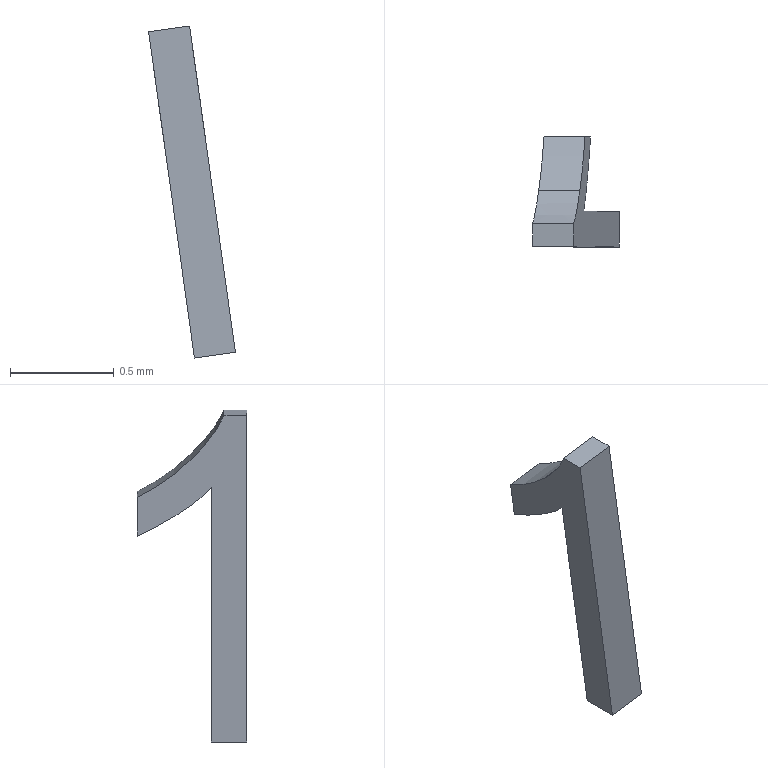Part | Creo | 1 solid | 11 faces | box 0.4191 x 0.529 x 1.601 mm | volume 0.06894 mm3 | plane 7 | other 4
STEP:
#1=CARTESIAN_POINT('',(-71.999,-126.498,-130.65));
#2=VERTEX_POINT('',#1);
#3=CARTESIAN_POINT('',(-72.171,-126.498,-129.425));
#4=VERTEX_POINT('',#3);
#5=CARTESIAN_POINT('',(-71.999,-126.498,-130.65));
#6=DIRECTION('',(-0.1392,0.,0.9903));
#7=VECTOR('',#6,1.237);
#8=LINE('',#5,#7);
#9=EDGE_CURVE('',#2,#4,#8,.T.);
#10=ORIENTED_EDGE('',*,*,#9,.F.);
#11=CARTESIAN_POINT('',(-71.801,-126.498,-130.622));
#12=VERTEX_POINT('',#11);
#13=CARTESIAN_POINT('',(-71.801,-126.498,-130.622));
#14=DIRECTION('',(-0.9903,0.,-0.1392));
#15=VECTOR('',#14,0.2);
#16=LINE('',#13,#15);
#17=EDGE_CURVE('',#12,#2,#16,.T.);
#18=ORIENTED_EDGE('',*,*,#17,.F.);
#19=CARTESIAN_POINT('',(-71.973,-126.498,-129.397));
#20=VERTEX_POINT('',#19);
#21=CARTESIAN_POINT('',(-71.973,-126.498,-129.397));
#22=DIRECTION('',(0.1392,0.,-0.9903));
#23=VECTOR('',#22,1.237);
#24=LINE('',#21,#23);
#25=EDGE_CURVE('',#20,#12,#24,.T.);
#26=ORIENTED_EDGE('',*,*,#25,.F.);
#27=CARTESIAN_POINT('',(-72.171,-126.498,-129.425));
#28=DIRECTION('',(0.9903,0.,0.1392));
#29=VECTOR('',#28,0.2);
#30=LINE('',#27,#29);
#31=EDGE_CURVE('',#4,#20,#30,.T.);
#32=ORIENTED_EDGE('',*,*,#31,.F.);
#33=EDGE_LOOP('',(#10,#18,#26,#32));
#34=FACE_OUTER_BOUND('',#33,.F.);
#35=CARTESIAN_POINT('',(-71.801,-126.498,-130.622));
#36=DIRECTION('',(0.,-1.,0.));
#37=DIRECTION('',(0.,0.,-1.));
#38=AXIS2_PLACEMENT_3D('',#35,#36,#37);
#39=PLANE('',#38);
#40=ADVANCED_FACE('',(#34),#39,.F.);
#41=ORIENTED_EDGE('',*,*,#9,.T.);
#42=CARTESIAN_POINT('',(-72.152,-126.328,-129.558));
#43=VERTEX_POINT('',#42);
#44=CARTESIAN_POINT('',(-72.154,-126.349,-129.545));
#45=CARTESIAN_POINT('',(-72.158,-126.388,-129.519));
#46=CARTESIAN_POINT('',(-72.164,-126.446,-129.476));
#47=CARTESIAN_POINT('',(-72.168,-126.481,-129.442));
#48=CARTESIAN_POINT('',(-72.171,-126.498,-129.425));
#49=B_SPLINE_CURVE_WITH_KNOTS('',3,(#42,#44,#45,#46,#47,#48),.UNSPECIFIED.,.F.,.F.,(4,1,1,4),(0.,0.3336,0.6671,1.),.UNSPECIFIED.);
#50=EDGE_CURVE('',#43,#4,#49,.T.);
#51=ORIENTED_EDGE('',*,*,#50,.F.);
#52=CARTESIAN_POINT('',(-72.138,-126.141,-129.657));
#53=VERTEX_POINT('',#52);
#54=CARTESIAN_POINT('',(-72.14,-126.163,-129.648));
#55=CARTESIAN_POINT('',(-72.142,-126.206,-129.629));
#56=CARTESIAN_POINT('',(-72.147,-126.268,-129.595));
#57=CARTESIAN_POINT('',(-72.15,-126.308,-129.571));
#58=CARTESIAN_POINT('',(-72.152,-126.328,-129.558));
#59=B_SPLINE_CURVE_WITH_KNOTS('',3,(#52,#54,#55,#56,#57,#58),.UNSPECIFIED.,.F.,.F.,(4,1,1,4),(0.,0.3335,0.6669,1.),.UNSPECIFIED.);
#60=EDGE_CURVE('',#53,#43,#59,.T.);
#61=ORIENTED_EDGE('',*,*,#60,.F.);
#62=CARTESIAN_POINT('',(-72.164,-126.141,-129.47));
#63=VERTEX_POINT('',#62);
#64=CARTESIAN_POINT('',(-72.138,-126.141,-129.657));
#65=DIRECTION('',(-0.1392,0.,0.9903));
#66=VECTOR('',#65,0.1886);
#67=LINE('',#64,#66);
#68=EDGE_CURVE('',#53,#63,#67,.T.);
#69=ORIENTED_EDGE('',*,*,#68,.T.);
#70=CARTESIAN_POINT('',(-72.19,-126.401,-129.288));
#71=VERTEX_POINT('',#70);
#72=CARTESIAN_POINT('',(-72.187,-126.375,-129.313));
#73=CARTESIAN_POINT('',(-72.18,-126.321,-129.36));
#74=CARTESIAN_POINT('',(-72.172,-126.234,-129.421));
#75=CARTESIAN_POINT('',(-72.167,-126.172,-129.455));
#76=CARTESIAN_POINT('',(-72.164,-126.141,-129.47));
#77=B_SPLINE_CURVE_WITH_KNOTS('',3,(#70,#72,#73,#74,#75,#76),.UNSPECIFIED.,.F.,.F.,(4,1,1,4),(0.,0.3333,0.6667,1.),.UNSPECIFIED.);
#78=EDGE_CURVE('',#71,#63,#77,.T.);
#79=ORIENTED_EDGE('',*,*,#78,.F.);
#80=CARTESIAN_POINT('',(-72.22,-126.559,-129.077));
#81=VERTEX_POINT('',#80);
#82=CARTESIAN_POINT('',(-72.216,-126.547,-129.105));
#83=CARTESIAN_POINT('',(-72.209,-126.518,-129.157));
#84=CARTESIAN_POINT('',(-72.199,-126.463,-129.226));
#85=CARTESIAN_POINT('',(-72.193,-126.422,-129.268));
#86=CARTESIAN_POINT('',(-72.19,-126.401,-129.288));
#87=B_SPLINE_CURVE_WITH_KNOTS('',3,(#80,#82,#83,#84,#85,#86),.UNSPECIFIED.,.F.,.F.,(4,1,1,4),(0.,0.3328,0.6668,1.),.UNSPECIFIED.);
#88=EDGE_CURVE('',#81,#71,#87,.T.);
#89=ORIENTED_EDGE('',*,*,#88,.F.);
#90=CARTESIAN_POINT('',(-72.22,-126.67,-129.077));
#91=VERTEX_POINT('',#90);
#92=CARTESIAN_POINT('',(-72.22,-126.67,-129.077));
#93=DIRECTION('',(0.,1.,0.));
#94=VECTOR('',#93,0.1108);
#95=LINE('',#92,#94);
#96=EDGE_CURVE('',#91,#81,#95,.T.);
#97=ORIENTED_EDGE('',*,*,#96,.F.);
#98=CARTESIAN_POINT('',(-71.999,-126.67,-130.65));
#99=VERTEX_POINT('',#98);
#100=CARTESIAN_POINT('',(-72.22,-126.67,-129.077));
#101=DIRECTION('',(0.1392,0.,-0.9903));
#102=VECTOR('',#101,1.589);
#103=LINE('',#100,#102);
#104=EDGE_CURVE('',#91,#99,#103,.T.);
#105=ORIENTED_EDGE('',*,*,#104,.T.);
#106=CARTESIAN_POINT('',(-71.999,-126.498,-130.65));
#107=DIRECTION('',(0.,-1.,0.));
#108=VECTOR('',#107,0.1716);
#109=LINE('',#106,#108);
#110=EDGE_CURVE('',#2,#99,#109,.T.);
#111=ORIENTED_EDGE('',*,*,#110,.F.);
#112=EDGE_LOOP('',(#41,#51,#61,#69,#79,#89,#97,#105,#111));
#113=FACE_OUTER_BOUND('',#112,.F.);
#114=CARTESIAN_POINT('',(-72.161,-126.417,-129.497));
#115=DIRECTION('',(-0.9903,0.,-0.1392));
#116=DIRECTION('',(-0.1392,0.,0.9903));
#117=AXIS2_PLACEMENT_3D('',#114,#115,#116);
#118=PLANE('',#117);
#119=ADVANCED_FACE('',(#113),#118,.T.);
#120=ORIENTED_EDGE('',*,*,#50,.T.);
#121=ORIENTED_EDGE('',*,*,#31,.T.);
#122=CARTESIAN_POINT('',(-71.954,-126.328,-129.53));
#123=VERTEX_POINT('',#122);
#124=CARTESIAN_POINT('',(-71.973,-126.498,-129.397));
#125=CARTESIAN_POINT('',(-71.97,-126.481,-129.414));
#126=CARTESIAN_POINT('',(-71.966,-126.446,-129.448));
#127=CARTESIAN_POINT('',(-71.96,-126.388,-129.491));
#128=CARTESIAN_POINT('',(-71.956,-126.349,-129.517));
#129=CARTESIAN_POINT('',(-71.954,-126.328,-129.53));
#130=B_SPLINE_CURVE_WITH_KNOTS('',3,(#124,#125,#126,#127,#128,#129),.UNSPECIFIED.,.F.,.F.,(4,1,1,4),(0.,0.3329,0.6664,1.),.UNSPECIFIED.);
#131=EDGE_CURVE('',#20,#123,#130,.T.);
#132=ORIENTED_EDGE('',*,*,#131,.T.);
#133=CARTESIAN_POINT('',(-72.152,-126.328,-129.558));
#134=DIRECTION('',(0.9903,0.,0.1392));
#135=VECTOR('',#134,0.2);
#136=LINE('',#133,#135);
#137=EDGE_CURVE('',#43,#123,#136,.T.);
#138=ORIENTED_EDGE('',*,*,#137,.F.);
#139=EDGE_LOOP('',(#120,#121,#132,#138));
#140=FACE_OUTER_BOUND('',#139,.F.);
#141=CARTESIAN_POINT('',(-71.973,-126.5,-129.395));
#142=CARTESIAN_POINT('',(-71.971,-126.482,-129.413));
#143=CARTESIAN_POINT('',(-71.966,-126.447,-129.447));
#144=CARTESIAN_POINT('',(-71.96,-126.388,-129.491));
#145=CARTESIAN_POINT('',(-71.956,-126.347,-129.518));
#146=CARTESIAN_POINT('',(-71.954,-126.326,-129.531));
#147=B_SPLINE_CURVE_WITH_KNOTS('',3,(#141,#142,#143,#144,#145,#146),.UNSPECIFIED.,.F.,.F.,(4,1,1,4),(0.,0.336,0.663,1.),.UNSPECIFIED.);
#148=DIRECTION('',(-0.9903,0.,-0.1392));
#149=VECTOR('',#148,1.);
#150=SURFACE_OF_LINEAR_EXTRUSION('',#147,#149);
#151=ADVANCED_FACE('',(#140),#150,.F.);
#152=ORIENTED_EDGE('',*,*,#25,.T.);
#153=CARTESIAN_POINT('',(-71.801,-126.67,-130.622));
#154=VERTEX_POINT('',#153);
#155=CARTESIAN_POINT('',(-71.801,-126.498,-130.622));
#156=DIRECTION('',(0.,-1.,0.));
#157=VECTOR('',#156,0.1716);
#158=LINE('',#155,#157);
#159=EDGE_CURVE('',#12,#154,#158,.T.);
#160=ORIENTED_EDGE('',*,*,#159,.T.);
#161=CARTESIAN_POINT('',(-72.022,-126.67,-129.049));
#162=VERTEX_POINT('',#161);
#163=CARTESIAN_POINT('',(-71.801,-126.67,-130.622));
#164=DIRECTION('',(-0.1392,0.,0.9903));
#165=VECTOR('',#164,1.589);
#166=LINE('',#163,#165);
#167=EDGE_CURVE('',#154,#162,#166,.T.);
#168=ORIENTED_EDGE('',*,*,#167,.T.);
#169=CARTESIAN_POINT('',(-72.022,-126.559,-129.049));
#170=VERTEX_POINT('',#169);
#171=CARTESIAN_POINT('',(-72.022,-126.67,-129.049));
#172=DIRECTION('',(0.,1.,0.));
#173=VECTOR('',#172,0.1108);
#174=LINE('',#171,#173);
#175=EDGE_CURVE('',#162,#170,#174,.T.);
#176=ORIENTED_EDGE('',*,*,#175,.T.);
#177=CARTESIAN_POINT('',(-71.992,-126.401,-129.26));
#178=VERTEX_POINT('',#177);
#179=CARTESIAN_POINT('',(-71.992,-126.401,-129.26));
#180=CARTESIAN_POINT('',(-71.995,-126.422,-129.24));
#181=CARTESIAN_POINT('',(-72.001,-126.463,-129.198));
#182=CARTESIAN_POINT('',(-72.011,-126.518,-129.129));
#183=CARTESIAN_POINT('',(-72.018,-126.547,-129.077));
#184=CARTESIAN_POINT('',(-72.022,-126.559,-129.049));
#185=B_SPLINE_CURVE_WITH_KNOTS('',3,(#179,#180,#181,#182,#183,#184),.UNSPECIFIED.,.F.,.F.,(4,1,1,4),(0.,0.3332,0.6672,1.),.UNSPECIFIED.);
#186=EDGE_CURVE('',#178,#170,#185,.T.);
#187=ORIENTED_EDGE('',*,*,#186,.F.);
#188=CARTESIAN_POINT('',(-71.966,-126.141,-129.443));
#189=VERTEX_POINT('',#188);
#190=CARTESIAN_POINT('',(-71.966,-126.141,-129.443));
#191=CARTESIAN_POINT('',(-71.969,-126.172,-129.427));
#192=CARTESIAN_POINT('',(-71.973,-126.234,-129.393));
#193=CARTESIAN_POINT('',(-71.982,-126.321,-129.332));
#194=CARTESIAN_POINT('',(-71.989,-126.375,-129.285));
#195=CARTESIAN_POINT('',(-71.992,-126.401,-129.26));
#196=B_SPLINE_CURVE_WITH_KNOTS('',3,(#190,#191,#192,#193,#194,#195),.UNSPECIFIED.,.F.,.F.,(4,1,1,4),(0.,0.3333,0.6667,1.),.UNSPECIFIED.);
#197=EDGE_CURVE('',#189,#178,#196,.T.);
#198=ORIENTED_EDGE('',*,*,#197,.F.);
#199=CARTESIAN_POINT('',(-71.94,-126.141,-129.629));
#200=VERTEX_POINT('',#199);
#201=CARTESIAN_POINT('',(-71.966,-126.141,-129.443));
#202=DIRECTION('',(0.1392,0.,-0.9903));
#203=VECTOR('',#202,0.1886);
#204=LINE('',#201,#203);
#205=EDGE_CURVE('',#189,#200,#204,.T.);
#206=ORIENTED_EDGE('',*,*,#205,.T.);
#207=CARTESIAN_POINT('',(-71.954,-126.328,-129.53));
#208=CARTESIAN_POINT('',(-71.952,-126.308,-129.543));
#209=CARTESIAN_POINT('',(-71.949,-126.268,-129.567));
#210=CARTESIAN_POINT('',(-71.944,-126.206,-129.601));
#211=CARTESIAN_POINT('',(-71.941,-126.163,-129.62));
#212=CARTESIAN_POINT('',(-71.94,-126.141,-129.629));
#213=B_SPLINE_CURVE_WITH_KNOTS('',3,(#207,#208,#209,#210,#211,#212),.UNSPECIFIED.,.F.,.F.,(4,1,1,4),(0.,0.3331,0.6665,1.),.UNSPECIFIED.);
#214=EDGE_CURVE('',#123,#200,#213,.T.);
#215=ORIENTED_EDGE('',*,*,#214,.F.);
#216=ORIENTED_EDGE('',*,*,#131,.F.);
#217=EDGE_LOOP('',(#152,#160,#168,#176,#187,#198,#206,#215,#216));
#218=FACE_OUTER_BOUND('',#217,.F.);
#219=CARTESIAN_POINT('',(-71.963,-126.417,-129.469));
#220=DIRECTION('',(-0.9903,0.,-0.1392));
#221=DIRECTION('',(-0.1392,0.,0.9903));
#222=AXIS2_PLACEMENT_3D('',#219,#220,#221);
#223=PLANE('',#222);
#224=ADVANCED_FACE('',(#218),#223,.F.);
#225=ORIENTED_EDGE('',*,*,#110,.T.);
#226=CARTESIAN_POINT('',(-71.999,-126.67,-130.65));
#227=DIRECTION('',(0.9903,0.,0.1392));
#228=VECTOR('',#227,0.2);
#229=LINE('',#226,#228);
#230=EDGE_CURVE('',#99,#154,#229,.T.);
#231=ORIENTED_EDGE('',*,*,#230,.T.);
#232=ORIENTED_EDGE('',*,*,#159,.F.);
#233=ORIENTED_EDGE('',*,*,#17,.T.);
#234=EDGE_LOOP('',(#225,#231,#232,#233));
#235=FACE_OUTER_BOUND('',#234,.F.);
#236=CARTESIAN_POINT('',(-71.801,-126.67,-130.622));
#237=DIRECTION('',(-0.1392,0.,0.9903));
#238=DIRECTION('',(0.9903,0.,0.1392));
#239=AXIS2_PLACEMENT_3D('',#236,#237,#238);
#240=PLANE('',#239);
#241=ADVANCED_FACE('',(#235),#240,.F.);
#242=ORIENTED_EDGE('',*,*,#104,.F.);
#243=CARTESIAN_POINT('',(-72.022,-126.67,-129.049));
#244=DIRECTION('',(-0.9903,0.,-0.1392));
#245=VECTOR('',#244,0.2);
#246=LINE('',#243,#245);
#247=EDGE_CURVE('',#162,#91,#246,.T.);
#248=ORIENTED_EDGE('',*,*,#247,.F.);
#249=ORIENTED_EDGE('',*,*,#167,.F.);
#250=ORIENTED_EDGE('',*,*,#230,.F.);
#251=EDGE_LOOP('',(#242,#248,#249,#250));
#252=FACE_OUTER_BOUND('',#251,.F.);
#253=CARTESIAN_POINT('',(-72.022,-126.67,-129.049));
#254=DIRECTION('',(0.,1.,0.));
#255=DIRECTION('',(0.,0.,1.));
#256=AXIS2_PLACEMENT_3D('',#253,#254,#255);
#257=PLANE('',#256);
#258=ADVANCED_FACE('',(#252),#257,.F.);
#259=ORIENTED_EDGE('',*,*,#96,.T.);
#260=CARTESIAN_POINT('',(-72.22,-126.559,-129.077));
#261=DIRECTION('',(0.9903,0.,0.1392));
#262=VECTOR('',#261,0.2);
#263=LINE('',#260,#262);
#264=EDGE_CURVE('',#81,#170,#263,.T.);
#265=ORIENTED_EDGE('',*,*,#264,.T.);
#266=ORIENTED_EDGE('',*,*,#175,.F.);
#267=ORIENTED_EDGE('',*,*,#247,.T.);
#268=EDGE_LOOP('',(#259,#265,#266,#267));
#269=FACE_OUTER_BOUND('',#268,.F.);
#270=CARTESIAN_POINT('',(-72.022,-126.559,-129.049));
#271=DIRECTION('',(0.1392,0.,-0.9903));
#272=DIRECTION('',(-0.9903,0.,-0.1392));
#273=AXIS2_PLACEMENT_3D('',#270,#271,#272);
#274=PLANE('',#273);
#275=ADVANCED_FACE('',(#269),#274,.F.);
#276=ORIENTED_EDGE('',*,*,#88,.T.);
#277=CARTESIAN_POINT('',(-72.19,-126.401,-129.288));
#278=DIRECTION('',(0.9903,0.,0.1392));
#279=VECTOR('',#278,0.2);
#280=LINE('',#277,#279);
#281=EDGE_CURVE('',#71,#178,#280,.T.);
#282=ORIENTED_EDGE('',*,*,#281,.T.);
#283=ORIENTED_EDGE('',*,*,#186,.T.);
#284=ORIENTED_EDGE('',*,*,#264,.F.);
#285=EDGE_LOOP('',(#276,#282,#283,#284));
#286=FACE_OUTER_BOUND('',#285,.F.);
#287=CARTESIAN_POINT('',(-71.992,-126.399,-129.262));
#288=CARTESIAN_POINT('',(-71.995,-126.421,-129.241));
#289=CARTESIAN_POINT('',(-72.001,-126.462,-129.199));
#290=CARTESIAN_POINT('',(-72.011,-126.518,-129.128));
#291=CARTESIAN_POINT('',(-72.018,-126.547,-129.075));
#292=CARTESIAN_POINT('',(-72.022,-126.56,-129.047));
#293=B_SPLINE_CURVE_WITH_KNOTS('',3,(#287,#288,#289,#290,#291,#292),.UNSPECIFIED.,.F.,.F.,(4,1,1,4),(0.,0.3367,0.6642,1.),.UNSPECIFIED.);
#294=DIRECTION('',(-0.9903,0.,-0.1392));
#295=VECTOR('',#294,1.);
#296=SURFACE_OF_LINEAR_EXTRUSION('',#293,#295);
#297=ADVANCED_FACE('',(#286),#296,.F.);
#298=ORIENTED_EDGE('',*,*,#78,.T.);
#299=CARTESIAN_POINT('',(-72.164,-126.141,-129.47));
#300=DIRECTION('',(0.9903,0.,0.1392));
#301=VECTOR('',#300,0.2);
#302=LINE('',#299,#301);
#303=EDGE_CURVE('',#63,#189,#302,.T.);
#304=ORIENTED_EDGE('',*,*,#303,.T.);
#305=ORIENTED_EDGE('',*,*,#197,.T.);
#306=ORIENTED_EDGE('',*,*,#281,.F.);
#307=EDGE_LOOP('',(#298,#304,#305,#306));
#308=FACE_OUTER_BOUND('',#307,.F.);
#309=CARTESIAN_POINT('',(-71.966,-126.138,-129.444));
#310=CARTESIAN_POINT('',(-71.968,-126.171,-129.428));
#311=CARTESIAN_POINT('',(-71.973,-126.233,-129.393));
#312=CARTESIAN_POINT('',(-71.982,-126.322,-129.332));
#313=CARTESIAN_POINT('',(-71.989,-126.377,-129.284));
#314=CARTESIAN_POINT('',(-71.992,-126.403,-129.258));
#315=B_SPLINE_CURVE_WITH_KNOTS('',3,(#309,#310,#311,#312,#313,#314),.UNSPECIFIED.,.F.,.F.,(4,1,1,4),(0.,0.3367,0.6636,1.),.UNSPECIFIED.);
#316=DIRECTION('',(-0.9903,0.,-0.1392));
#317=VECTOR('',#316,1.);
#318=SURFACE_OF_LINEAR_EXTRUSION('',#315,#317);
#319=ADVANCED_FACE('',(#308),#318,.F.);
#320=ORIENTED_EDGE('',*,*,#68,.F.);
#321=CARTESIAN_POINT('',(-71.94,-126.141,-129.629));
#322=DIRECTION('',(-0.9903,0.,-0.1392));
#323=VECTOR('',#322,0.2);
#324=LINE('',#321,#323);
#325=EDGE_CURVE('',#200,#53,#324,.T.);
#326=ORIENTED_EDGE('',*,*,#325,.F.);
#327=ORIENTED_EDGE('',*,*,#205,.F.);
#328=ORIENTED_EDGE('',*,*,#303,.F.);
#329=EDGE_LOOP('',(#320,#326,#327,#328));
#330=FACE_OUTER_BOUND('',#329,.F.);
#331=CARTESIAN_POINT('',(-71.94,-126.141,-129.629));
#332=DIRECTION('',(0.,-1.,0.));
#333=DIRECTION('',(0.,0.,-1.));
#334=AXIS2_PLACEMENT_3D('',#331,#332,#333);
#335=PLANE('',#334);
#336=ADVANCED_FACE('',(#330),#335,.F.);
#337=ORIENTED_EDGE('',*,*,#60,.T.);
#338=ORIENTED_EDGE('',*,*,#137,.T.);
#339=ORIENTED_EDGE('',*,*,#214,.T.);
#340=ORIENTED_EDGE('',*,*,#325,.T.);
#341=EDGE_LOOP('',(#337,#338,#339,#340));
#342=FACE_OUTER_BOUND('',#341,.F.);
#343=CARTESIAN_POINT('',(-71.954,-126.33,-129.529));
#344=CARTESIAN_POINT('',(-71.952,-126.31,-129.542));
#345=CARTESIAN_POINT('',(-71.949,-126.268,-129.567));
#346=CARTESIAN_POINT('',(-71.944,-126.205,-129.602));
#347=CARTESIAN_POINT('',(-71.941,-126.161,-129.621));
#348=CARTESIAN_POINT('',(-71.94,-126.139,-129.63));
#349=B_SPLINE_CURVE_WITH_KNOTS('',3,(#343,#344,#345,#346,#347,#348),.UNSPECIFIED.,.F.,.F.,(4,1,1,4),(0.,0.3362,0.6632,1.),.UNSPECIFIED.);
#350=DIRECTION('',(-0.9903,0.,-0.1392));
#351=VECTOR('',#350,1.);
#352=SURFACE_OF_LINEAR_EXTRUSION('',#349,#351);
#353=ADVANCED_FACE('',(#342),#352,.F.);
#354=CLOSED_SHELL('',(#40,#119,#151,#224,#241,#258,#275,#297,#319,#336,#353));
#355=MANIFOLD_SOLID_BREP('',#354);
#356=(LENGTH_UNIT()NAMED_UNIT(*)SI_UNIT(.MILLI.,.METRE.));
#357=UNCERTAINTY_MEASURE_WITH_UNIT(LENGTH_MEASURE(0.0001737),#356,'','');
#358=(NAMED_UNIT(*)PLANE_ANGLE_UNIT()SI_UNIT($,.RADIAN.));
#359=PLANE_ANGLE_MEASURE_WITH_UNIT(PLANE_ANGLE_MEASURE(0.01745),#358);
#360=(CONVERSION_BASED_UNIT('DEGREE',#359)NAMED_UNIT(*)PLANE_ANGLE_UNIT());
#361=(NAMED_UNIT(*)SI_UNIT($,.STERADIAN.)SOLID_ANGLE_UNIT());
#362=(GEOMETRIC_REPRESENTATION_CONTEXT(3)GLOBAL_UNCERTAINTY_ASSIGNED_CONTEXT((#357))GLOBAL_UNIT_ASSIGNED_CONTEXT((#356,#360,#361))REPRESENTATION_CONTEXT('',''));
#363=ADVANCED_BREP_SHAPE_REPRESENTATION('',(#355),#362);